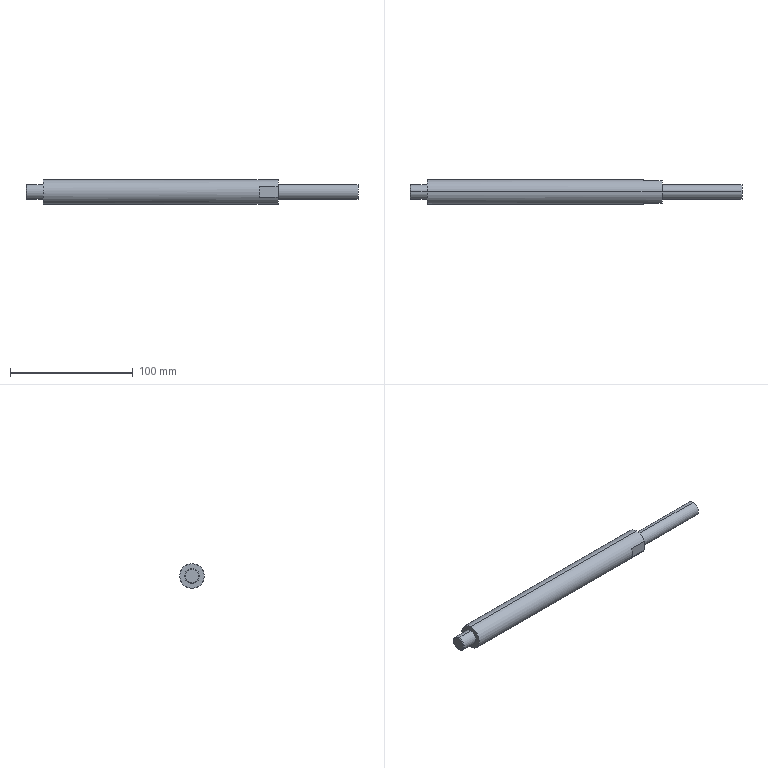Part | SolidWorks | features ICE 2, Chamfer 1, Revolution 1 | 1 solid | 16 faces | box 270 x 20 x 20 mm | volume 68758 mm3 | plane 8 | cylinder 6 | cone 2 | commonest cylinder face diameters 12 x4 20 x2
STEP:
#1=CARTESIAN_POINT('',(-14.,0.,5.5));
#2=VERTEX_POINT('',#1);
#3=CARTESIAN_POINT('',(-14.,0.,-5.5));
#4=VERTEX_POINT('',#3);
#5=CARTESIAN_POINT('',(-14.,0.,0.));
#6=DIRECTION('',(-1.,0.,0.));
#7=DIRECTION('',(0.,0.,1.));
#8=AXIS2_PLACEMENT_3D('',#5,#6,#7);
#9=CIRCLE('',#8,5.5);
#10=EDGE_CURVE('',#2,#4,#9,.T.);
#11=ORIENTED_EDGE('',*,*,#10,.F.);
#12=CARTESIAN_POINT('',(-13.5,0.,6.));
#13=VERTEX_POINT('',#12);
#14=CARTESIAN_POINT('',(-14.,0.,5.5));
#15=DIRECTION('',(0.7071,0.,0.7071));
#16=VECTOR('',#15,1000.);
#17=LINE('',#14,#16);
#18=EDGE_CURVE('',#2,#13,#17,.T.);
#19=ORIENTED_EDGE('',*,*,#18,.T.);
#20=CARTESIAN_POINT('',(-13.5,0.,-6.));
#21=VERTEX_POINT('',#20);
#22=CARTESIAN_POINT('',(-13.5,0.,0.));
#23=DIRECTION('',(1.,0.,0.));
#24=DIRECTION('',(0.,0.,1.));
#25=AXIS2_PLACEMENT_3D('',#22,#23,#24);
#26=CIRCLE('',#25,6.);
#27=EDGE_CURVE('',#21,#13,#26,.T.);
#28=ORIENTED_EDGE('',*,*,#27,.F.);
#29=CARTESIAN_POINT('',(-14.,0.,-5.5));
#30=DIRECTION('',(0.7071,0.,-0.7071));
#31=VECTOR('',#30,1000.);
#32=LINE('',#29,#31);
#33=EDGE_CURVE('',#4,#21,#32,.T.);
#34=ORIENTED_EDGE('',*,*,#33,.F.);
#35=EDGE_LOOP('',(#11,#19,#28,#34));
#36=FACE_OUTER_BOUND('',#35,.T.);
#37=CARTESIAN_POINT('',(-14.,0.,0.));
#38=DIRECTION('',(1.,0.,0.));
#39=DIRECTION('',(0.,0.,-1.));
#40=AXIS2_PLACEMENT_3D('',#37,#38,#39);
#41=CONICAL_SURFACE('',#40,5.5,0.7854);
#42=ADVANCED_FACE('',(#36),#41,.T.);
#43=ORIENTED_EDGE('',*,*,#27,.T.);
#44=CARTESIAN_POINT('',(0.,0.,6.));
#45=VERTEX_POINT('',#44);
#46=CARTESIAN_POINT('',(-14.,0.,6.));
#47=DIRECTION('',(1.,0.,0.));
#48=VECTOR('',#47,1000.);
#49=LINE('',#46,#48);
#50=EDGE_CURVE('',#13,#45,#49,.T.);
#51=ORIENTED_EDGE('',*,*,#50,.T.);
#52=CARTESIAN_POINT('',(0.,0.,-6.));
#53=VERTEX_POINT('',#52);
#54=CARTESIAN_POINT('',(0.,0.,0.));
#55=DIRECTION('',(-1.,0.,0.));
#56=DIRECTION('',(0.,0.,1.));
#57=AXIS2_PLACEMENT_3D('',#54,#55,#56);
#58=CIRCLE('',#57,6.);
#59=EDGE_CURVE('',#45,#53,#58,.T.);
#60=ORIENTED_EDGE('',*,*,#59,.T.);
#61=CARTESIAN_POINT('',(-14.,0.,-6.));
#62=DIRECTION('',(1.,0.,0.));
#63=VECTOR('',#62,1000.);
#64=LINE('',#61,#63);
#65=EDGE_CURVE('',#21,#53,#64,.T.);
#66=ORIENTED_EDGE('',*,*,#65,.F.);
#67=EDGE_LOOP('',(#43,#51,#60,#66));
#68=FACE_OUTER_BOUND('',#67,.T.);
#69=CARTESIAN_POINT('',(-14.,0.,0.));
#70=DIRECTION('',(1.,0.,0.));
#71=DIRECTION('',(0.,0.,-1.));
#72=AXIS2_PLACEMENT_3D('',#69,#70,#71);
#73=CYLINDRICAL_SURFACE('',#72,6.);
#74=ADVANCED_FACE('',(#68),#73,.T.);
#75=CARTESIAN_POINT('',(256.,0.,6.));
#76=VERTEX_POINT('',#75);
#77=CARTESIAN_POINT('',(256.,0.,-6.));
#78=VERTEX_POINT('',#77);
#79=CARTESIAN_POINT('',(256.,0.,0.));
#80=DIRECTION('',(-1.,0.,0.));
#81=DIRECTION('',(0.,0.,1.));
#82=AXIS2_PLACEMENT_3D('',#79,#80,#81);
#83=CIRCLE('',#82,6.);
#84=EDGE_CURVE('',#76,#78,#83,.T.);
#85=ORIENTED_EDGE('',*,*,#84,.T.);
#86=CARTESIAN_POINT('',(191.,0.,-6.));
#87=VERTEX_POINT('',#86);
#88=CARTESIAN_POINT('',(0.,0.,-6.));
#89=DIRECTION('',(-1.,0.,0.));
#90=VECTOR('',#89,1000.);
#91=LINE('',#88,#90);
#92=EDGE_CURVE('',#78,#87,#91,.T.);
#93=ORIENTED_EDGE('',*,*,#92,.T.);
#94=CARTESIAN_POINT('',(191.,0.,6.));
#95=VERTEX_POINT('',#94);
#96=CARTESIAN_POINT('',(191.,0.,0.));
#97=DIRECTION('',(-1.,0.,0.));
#98=DIRECTION('',(0.,0.,1.));
#99=AXIS2_PLACEMENT_3D('',#96,#97,#98);
#100=CIRCLE('',#99,6.);
#101=EDGE_CURVE('',#95,#87,#100,.T.);
#102=ORIENTED_EDGE('',*,*,#101,.F.);
#103=CARTESIAN_POINT('',(0.,0.,6.));
#104=DIRECTION('',(-1.,0.,0.));
#105=VECTOR('',#104,1000.);
#106=LINE('',#103,#105);
#107=EDGE_CURVE('',#76,#95,#106,.T.);
#108=ORIENTED_EDGE('',*,*,#107,.F.);
#109=EDGE_LOOP('',(#85,#93,#102,#108));
#110=FACE_OUTER_BOUND('',#109,.T.);
#111=CARTESIAN_POINT('',(0.,0.,0.));
#112=DIRECTION('',(-1.,0.,0.));
#113=DIRECTION('',(0.,0.,1.));
#114=AXIS2_PLACEMENT_3D('',#111,#112,#113);
#115=CYLINDRICAL_SURFACE('',#114,6.);
#116=ADVANCED_FACE('',(#110),#115,.T.);
#117=CARTESIAN_POINT('',(191.,9.,-4.359));
#118=VERTEX_POINT('',#117);
#119=CARTESIAN_POINT('',(191.,0.,-10.));
#120=VERTEX_POINT('',#119);
#121=CARTESIAN_POINT('',(191.,0.,0.));
#122=DIRECTION('',(-1.,0.,0.));
#123=DIRECTION('',(0.,0.,1.));
#124=AXIS2_PLACEMENT_3D('',#121,#122,#123);
#125=CIRCLE('',#124,10.);
#126=EDGE_CURVE('',#118,#120,#125,.T.);
#127=ORIENTED_EDGE('',*,*,#126,.T.);
#128=CARTESIAN_POINT('',(0.,0.,-10.));
#129=VERTEX_POINT('',#128);
#130=CARTESIAN_POINT('',(0.,0.,-10.));
#131=DIRECTION('',(-1.,0.,0.));
#132=VECTOR('',#131,1000.);
#133=LINE('',#130,#132);
#134=EDGE_CURVE('',#120,#129,#133,.T.);
#135=ORIENTED_EDGE('',*,*,#134,.T.);
#136=CARTESIAN_POINT('',(0.,0.,10.));
#137=VERTEX_POINT('',#136);
#138=CARTESIAN_POINT('',(0.,0.,0.));
#139=DIRECTION('',(-1.,0.,0.));
#140=DIRECTION('',(0.,0.,1.));
#141=AXIS2_PLACEMENT_3D('',#138,#139,#140);
#142=CIRCLE('',#141,10.);
#143=EDGE_CURVE('',#137,#129,#142,.T.);
#144=ORIENTED_EDGE('',*,*,#143,.F.);
#145=CARTESIAN_POINT('',(191.,0.,10.));
#146=VERTEX_POINT('',#145);
#147=CARTESIAN_POINT('',(0.,0.,10.));
#148=DIRECTION('',(-1.,0.,0.));
#149=VECTOR('',#148,1000.);
#150=LINE('',#147,#149);
#151=EDGE_CURVE('',#146,#137,#150,.T.);
#152=ORIENTED_EDGE('',*,*,#151,.F.);
#153=CARTESIAN_POINT('',(191.,9.,4.359));
#154=VERTEX_POINT('',#153);
#155=CARTESIAN_POINT('',(191.,0.,0.));
#156=DIRECTION('',(-1.,0.,0.));
#157=DIRECTION('',(0.,0.,1.));
#158=AXIS2_PLACEMENT_3D('',#155,#156,#157);
#159=CIRCLE('',#158,10.);
#160=EDGE_CURVE('',#146,#154,#159,.T.);
#161=ORIENTED_EDGE('',*,*,#160,.T.);
#162=CARTESIAN_POINT('',(176.,9.,4.359));
#163=VERTEX_POINT('',#162);
#164=CARTESIAN_POINT('',(0.,9.,4.359));
#165=DIRECTION('',(-1.,0.,0.));
#166=VECTOR('',#165,1000.);
#167=LINE('',#164,#166);
#168=EDGE_CURVE('',#154,#163,#167,.T.);
#169=ORIENTED_EDGE('',*,*,#168,.T.);
#170=CARTESIAN_POINT('',(176.,9.,-4.359));
#171=VERTEX_POINT('',#170);
#172=CARTESIAN_POINT('',(176.,0.,0.));
#173=DIRECTION('',(-1.,0.,0.));
#174=DIRECTION('',(0.,0.,1.));
#175=AXIS2_PLACEMENT_3D('',#172,#173,#174);
#176=CIRCLE('',#175,10.);
#177=EDGE_CURVE('',#163,#171,#176,.T.);
#178=ORIENTED_EDGE('',*,*,#177,.T.);
#179=CARTESIAN_POINT('',(0.,9.,-4.359));
#180=DIRECTION('',(1.,0.,0.));
#181=VECTOR('',#180,1000.);
#182=LINE('',#179,#181);
#183=EDGE_CURVE('',#171,#118,#182,.T.);
#184=ORIENTED_EDGE('',*,*,#183,.T.);
#185=EDGE_LOOP('',(#127,#135,#144,#152,#161,#169,#178,#184));
#186=FACE_OUTER_BOUND('',#185,.T.);
#187=CARTESIAN_POINT('',(0.,0.,0.));
#188=DIRECTION('',(-1.,0.,0.));
#189=DIRECTION('',(0.,0.,1.));
#190=AXIS2_PLACEMENT_3D('',#187,#188,#189);
#191=CYLINDRICAL_SURFACE('',#190,10.);
#192=ADVANCED_FACE('',(#186),#191,.T.);
#193=CARTESIAN_POINT('',(0.,0.,0.));
#194=DIRECTION('',(-1.,0.,0.));
#195=DIRECTION('',(0.,0.,1.));
#196=AXIS2_PLACEMENT_3D('',#193,#194,#195);
#197=CIRCLE('',#196,6.);
#198=EDGE_CURVE('',#53,#45,#197,.T.);
#199=ORIENTED_EDGE('',*,*,#198,.F.);
#200=ORIENTED_EDGE('',*,*,#59,.F.);
#201=EDGE_LOOP('',(#199,#200));
#202=FACE_BOUND('',#201,.T.);
#203=ORIENTED_EDGE('',*,*,#143,.T.);
#204=CARTESIAN_POINT('',(0.,0.,0.));
#205=DIRECTION('',(-1.,0.,0.));
#206=DIRECTION('',(0.,0.,1.));
#207=AXIS2_PLACEMENT_3D('',#204,#205,#206);
#208=CIRCLE('',#207,10.);
#209=EDGE_CURVE('',#129,#137,#208,.T.);
#210=ORIENTED_EDGE('',*,*,#209,.T.);
#211=EDGE_LOOP('',(#203,#210));
#212=FACE_OUTER_BOUND('',#211,.T.);
#213=CARTESIAN_POINT('',(0.,0.,0.));
#214=DIRECTION('',(1.,0.,0.));
#215=DIRECTION('',(0.,0.,-1.));
#216=AXIS2_PLACEMENT_3D('',#213,#214,#215);
#217=PLANE('',#216);
#218=ADVANCED_FACE('',(#202,#212),#217,.F.);
#219=ORIENTED_EDGE('',*,*,#134,.F.);
#220=CARTESIAN_POINT('',(191.,-9.,-4.359));
#221=VERTEX_POINT('',#220);
#222=CARTESIAN_POINT('',(191.,0.,0.));
#223=DIRECTION('',(-1.,0.,0.));
#224=DIRECTION('',(0.,0.,1.));
#225=AXIS2_PLACEMENT_3D('',#222,#223,#224);
#226=CIRCLE('',#225,10.);
#227=EDGE_CURVE('',#120,#221,#226,.T.);
#228=ORIENTED_EDGE('',*,*,#227,.T.);
#229=CARTESIAN_POINT('',(176.,-9.,-4.359));
#230=VERTEX_POINT('',#229);
#231=CARTESIAN_POINT('',(0.,-9.,-4.359));
#232=DIRECTION('',(-1.,0.,0.));
#233=VECTOR('',#232,1000.);
#234=LINE('',#231,#233);
#235=EDGE_CURVE('',#221,#230,#234,.T.);
#236=ORIENTED_EDGE('',*,*,#235,.T.);
#237=CARTESIAN_POINT('',(176.,-9.,4.359));
#238=VERTEX_POINT('',#237);
#239=CARTESIAN_POINT('',(176.,0.,0.));
#240=DIRECTION('',(-1.,0.,0.));
#241=DIRECTION('',(0.,0.,1.));
#242=AXIS2_PLACEMENT_3D('',#239,#240,#241);
#243=CIRCLE('',#242,10.);
#244=EDGE_CURVE('',#230,#238,#243,.T.);
#245=ORIENTED_EDGE('',*,*,#244,.T.);
#246=CARTESIAN_POINT('',(191.,-9.,4.359));
#247=VERTEX_POINT('',#246);
#248=CARTESIAN_POINT('',(0.,-9.,4.359));
#249=DIRECTION('',(1.,0.,0.));
#250=VECTOR('',#249,1000.);
#251=LINE('',#248,#250);
#252=EDGE_CURVE('',#238,#247,#251,.T.);
#253=ORIENTED_EDGE('',*,*,#252,.T.);
#254=CARTESIAN_POINT('',(191.,0.,0.));
#255=DIRECTION('',(-1.,0.,0.));
#256=DIRECTION('',(0.,0.,1.));
#257=AXIS2_PLACEMENT_3D('',#254,#255,#256);
#258=CIRCLE('',#257,10.);
#259=EDGE_CURVE('',#247,#146,#258,.T.);
#260=ORIENTED_EDGE('',*,*,#259,.T.);
#261=ORIENTED_EDGE('',*,*,#151,.T.);
#262=ORIENTED_EDGE('',*,*,#209,.F.);
#263=EDGE_LOOP('',(#219,#228,#236,#245,#253,#260,#261,#262));
#264=FACE_OUTER_BOUND('',#263,.T.);
#265=CARTESIAN_POINT('',(0.,0.,0.));
#266=DIRECTION('',(-1.,0.,0.));
#267=DIRECTION('',(0.,0.,1.));
#268=AXIS2_PLACEMENT_3D('',#265,#266,#267);
#269=CYLINDRICAL_SURFACE('',#268,10.);
#270=ADVANCED_FACE('',(#264),#269,.T.);
#271=ORIENTED_EDGE('',*,*,#126,.F.);
#272=CARTESIAN_POINT('',(191.,9.,0.));
#273=DIRECTION('',(0.,0.,1.));
#274=VECTOR('',#273,1000.);
#275=LINE('',#272,#274);
#276=EDGE_CURVE('',#118,#154,#275,.T.);
#277=ORIENTED_EDGE('',*,*,#276,.T.);
#278=ORIENTED_EDGE('',*,*,#160,.F.);
#279=ORIENTED_EDGE('',*,*,#259,.F.);
#280=CARTESIAN_POINT('',(191.,-9.,0.));
#281=DIRECTION('',(0.,0.,-1.));
#282=VECTOR('',#281,1000.);
#283=LINE('',#280,#282);
#284=EDGE_CURVE('',#247,#221,#283,.T.);
#285=ORIENTED_EDGE('',*,*,#284,.T.);
#286=ORIENTED_EDGE('',*,*,#227,.F.);
#287=EDGE_LOOP('',(#271,#277,#278,#279,#285,#286));
#288=FACE_OUTER_BOUND('',#287,.T.);
#289=ORIENTED_EDGE('',*,*,#101,.T.);
#290=CARTESIAN_POINT('',(191.,0.,0.));
#291=DIRECTION('',(-1.,0.,0.));
#292=DIRECTION('',(0.,0.,1.));
#293=AXIS2_PLACEMENT_3D('',#290,#291,#292);
#294=CIRCLE('',#293,6.);
#295=EDGE_CURVE('',#87,#95,#294,.T.);
#296=ORIENTED_EDGE('',*,*,#295,.T.);
#297=EDGE_LOOP('',(#289,#296));
#298=FACE_BOUND('',#297,.T.);
#299=CARTESIAN_POINT('',(191.,10.,0.));
#300=DIRECTION('',(-1.,0.,0.));
#301=DIRECTION('',(0.,0.,1.));
#302=AXIS2_PLACEMENT_3D('',#299,#300,#301);
#303=PLANE('',#302);
#304=ADVANCED_FACE('',(#288,#298),#303,.F.);
#305=ORIENTED_EDGE('',*,*,#92,.F.);
#306=CARTESIAN_POINT('',(256.,0.,0.));
#307=DIRECTION('',(-1.,0.,0.));
#308=DIRECTION('',(0.,0.,1.));
#309=AXIS2_PLACEMENT_3D('',#306,#307,#308);
#310=CIRCLE('',#309,6.);
#311=EDGE_CURVE('',#78,#76,#310,.T.);
#312=ORIENTED_EDGE('',*,*,#311,.T.);
#313=ORIENTED_EDGE('',*,*,#107,.T.);
#314=ORIENTED_EDGE('',*,*,#295,.F.);
#315=EDGE_LOOP('',(#305,#312,#313,#314));
#316=FACE_OUTER_BOUND('',#315,.T.);
#317=CARTESIAN_POINT('',(0.,0.,0.));
#318=DIRECTION('',(-1.,0.,0.));
#319=DIRECTION('',(0.,0.,1.));
#320=AXIS2_PLACEMENT_3D('',#317,#318,#319);
#321=CYLINDRICAL_SURFACE('',#320,6.);
#322=ADVANCED_FACE('',(#316),#321,.T.);
#323=ORIENTED_EDGE('',*,*,#84,.F.);
#324=ORIENTED_EDGE('',*,*,#311,.F.);
#325=EDGE_LOOP('',(#323,#324));
#326=FACE_OUTER_BOUND('',#325,.T.);
#327=CARTESIAN_POINT('',(256.,6.,0.));
#328=DIRECTION('',(-1.,0.,0.));
#329=DIRECTION('',(0.,0.,1.));
#330=AXIS2_PLACEMENT_3D('',#327,#328,#329);
#331=PLANE('',#330);
#332=ADVANCED_FACE('',(#326),#331,.F.);
#333=ORIENTED_EDGE('',*,*,#50,.F.);
#334=CARTESIAN_POINT('',(-13.5,0.,0.));
#335=DIRECTION('',(1.,0.,0.));
#336=DIRECTION('',(0.,0.,1.));
#337=AXIS2_PLACEMENT_3D('',#334,#335,#336);
#338=CIRCLE('',#337,6.);
#339=EDGE_CURVE('',#13,#21,#338,.T.);
#340=ORIENTED_EDGE('',*,*,#339,.T.);
#341=ORIENTED_EDGE('',*,*,#65,.T.);
#342=ORIENTED_EDGE('',*,*,#198,.T.);
#343=EDGE_LOOP('',(#333,#340,#341,#342));
#344=FACE_OUTER_BOUND('',#343,.T.);
#345=CARTESIAN_POINT('',(-14.,0.,0.));
#346=DIRECTION('',(1.,0.,0.));
#347=DIRECTION('',(0.,0.,-1.));
#348=AXIS2_PLACEMENT_3D('',#345,#346,#347);
#349=CYLINDRICAL_SURFACE('',#348,6.);
#350=ADVANCED_FACE('',(#344),#349,.T.);
#351=CARTESIAN_POINT('',(-14.,0.,0.));
#352=DIRECTION('',(-1.,0.,0.));
#353=DIRECTION('',(0.,0.,1.));
#354=AXIS2_PLACEMENT_3D('',#351,#352,#353);
#355=CIRCLE('',#354,5.5);
#356=EDGE_CURVE('',#4,#2,#355,.T.);
#357=ORIENTED_EDGE('',*,*,#356,.T.);
#358=ORIENTED_EDGE('',*,*,#10,.T.);
#359=EDGE_LOOP('',(#357,#358));
#360=FACE_OUTER_BOUND('',#359,.T.);
#361=CARTESIAN_POINT('',(-14.,0.,0.));
#362=DIRECTION('',(-1.,0.,0.));
#363=DIRECTION('',(0.,0.,1.));
#364=AXIS2_PLACEMENT_3D('',#361,#362,#363);
#365=PLANE('',#364);
#366=ADVANCED_FACE('',(#360),#365,.T.);
#367=ORIENTED_EDGE('',*,*,#18,.F.);
#368=ORIENTED_EDGE('',*,*,#356,.F.);
#369=ORIENTED_EDGE('',*,*,#33,.T.);
#370=ORIENTED_EDGE('',*,*,#339,.F.);
#371=EDGE_LOOP('',(#367,#368,#369,#370));
#372=FACE_OUTER_BOUND('',#371,.T.);
#373=CARTESIAN_POINT('',(-14.,0.,0.));
#374=DIRECTION('',(1.,0.,0.));
#375=DIRECTION('',(0.,0.,-1.));
#376=AXIS2_PLACEMENT_3D('',#373,#374,#375);
#377=CONICAL_SURFACE('',#376,5.5,0.7854);
#378=ADVANCED_FACE('',(#372),#377,.T.);
#379=CARTESIAN_POINT('',(176.,-9.,-10.));
#380=DIRECTION('',(0.,0.,1.));
#381=VECTOR('',#380,1000.);
#382=LINE('',#379,#381);
#383=EDGE_CURVE('',#230,#238,#382,.T.);
#384=ORIENTED_EDGE('',*,*,#383,.T.);
#385=ORIENTED_EDGE('',*,*,#244,.F.);
#386=EDGE_LOOP('',(#384,#385));
#387=FACE_OUTER_BOUND('',#386,.T.);
#388=CARTESIAN_POINT('',(176.,-10.,-10.));
#389=DIRECTION('',(-1.,0.,0.));
#390=DIRECTION('',(0.,0.,1.));
#391=AXIS2_PLACEMENT_3D('',#388,#389,#390);
#392=PLANE('',#391);
#393=ADVANCED_FACE('',(#387),#392,.F.);
#394=ORIENTED_EDGE('',*,*,#284,.F.);
#395=ORIENTED_EDGE('',*,*,#252,.F.);
#396=ORIENTED_EDGE('',*,*,#383,.F.);
#397=ORIENTED_EDGE('',*,*,#235,.F.);
#398=EDGE_LOOP('',(#394,#395,#396,#397));
#399=FACE_OUTER_BOUND('',#398,.T.);
#400=CARTESIAN_POINT('',(191.,-9.,-10.));
#401=DIRECTION('',(0.,1.,0.));
#402=DIRECTION('',(-1.,0.,0.));
#403=AXIS2_PLACEMENT_3D('',#400,#401,#402);
#404=PLANE('',#403);
#405=ADVANCED_FACE('',(#399),#404,.F.);
#406=CARTESIAN_POINT('',(176.,9.,-10.));
#407=DIRECTION('',(0.,0.,1.));
#408=VECTOR('',#407,1000.);
#409=LINE('',#406,#408);
#410=EDGE_CURVE('',#171,#163,#409,.T.);
#411=ORIENTED_EDGE('',*,*,#410,.F.);
#412=ORIENTED_EDGE('',*,*,#177,.F.);
#413=EDGE_LOOP('',(#411,#412));
#414=FACE_OUTER_BOUND('',#413,.T.);
#415=CARTESIAN_POINT('',(176.,10.,-10.));
#416=DIRECTION('',(-1.,0.,0.));
#417=DIRECTION('',(0.,0.,1.));
#418=AXIS2_PLACEMENT_3D('',#415,#416,#417);
#419=PLANE('',#418);
#420=ADVANCED_FACE('',(#414),#419,.F.);
#421=ORIENTED_EDGE('',*,*,#276,.F.);
#422=ORIENTED_EDGE('',*,*,#183,.F.);
#423=ORIENTED_EDGE('',*,*,#410,.T.);
#424=ORIENTED_EDGE('',*,*,#168,.F.);
#425=EDGE_LOOP('',(#421,#422,#423,#424));
#426=FACE_OUTER_BOUND('',#425,.T.);
#427=CARTESIAN_POINT('',(191.,9.,-10.));
#428=DIRECTION('',(0.,-1.,0.));
#429=DIRECTION('',(1.,0.,0.));
#430=AXIS2_PLACEMENT_3D('',#427,#428,#429);
#431=PLANE('',#430);
#432=ADVANCED_FACE('',(#426),#431,.F.);
#433=CLOSED_SHELL('',(#42,#74,#116,#192,#218,#270,#304,#322,#332,#350,#366,#378,#393,#405,#420,#432));
#434=MANIFOLD_SOLID_BREP('',#433);
#435=CARTESIAN_POINT('',(0.,0.,0.));
#436=DIRECTION('',(0.,0.,1.));
#437=DIRECTION('',(1.,0.,0.));
#438=AXIS2_PLACEMENT_3D('',#435,#436,#437);
#439=(LENGTH_UNIT()NAMED_UNIT(*)SI_UNIT(.MILLI.,.METRE.));
#440=UNCERTAINTY_MEASURE_WITH_UNIT(LENGTH_MEASURE(0.00001),#439,'','');
#441=(NAMED_UNIT(*)PLANE_ANGLE_UNIT()SI_UNIT($,.RADIAN.));
#442=(NAMED_UNIT(*)SI_UNIT($,.STERADIAN.)SOLID_ANGLE_UNIT());
#443=(GEOMETRIC_REPRESENTATION_CONTEXT(3)GLOBAL_UNCERTAINTY_ASSIGNED_CONTEXT((#440))GLOBAL_UNIT_ASSIGNED_CONTEXT((#439,#441,#442))REPRESENTATION_CONTEXT('',''));
#444=ADVANCED_BREP_SHAPE_REPRESENTATION('',(#434,#438),#443);